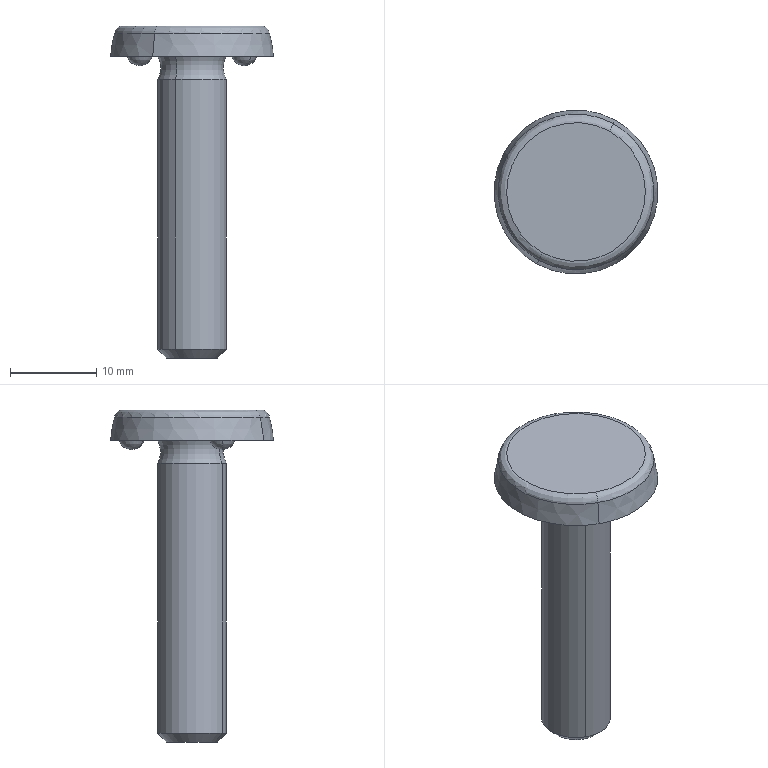Part | 1 solid | 19 faces | box 19 x 19 x 38.5 mm | volume 2667 mm3 | sphere 6 | cone 4 | torus 4 | plane 3 | cylinder 2 | commonest cylinder face diameters 8 x2